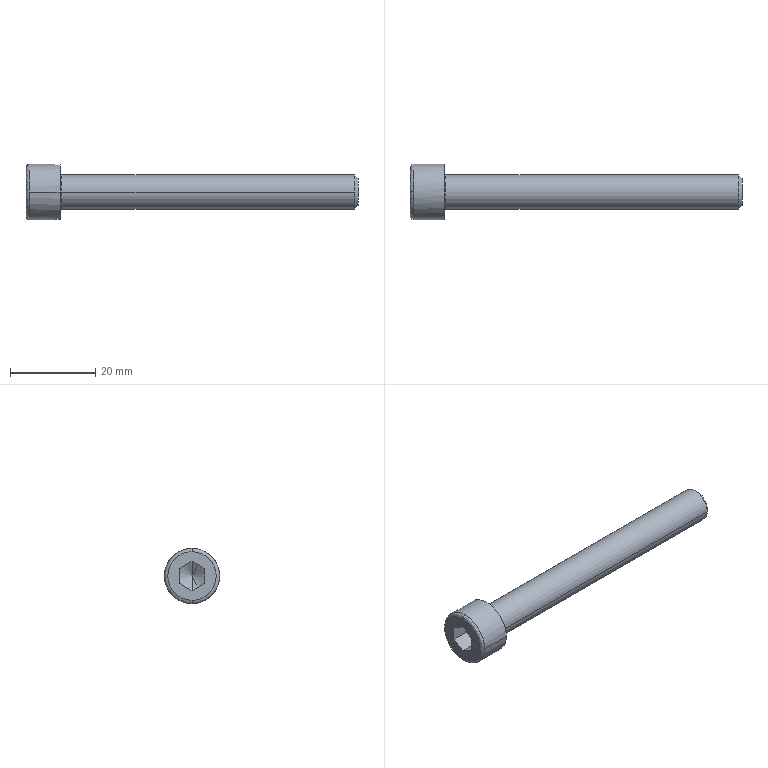Part | STEP file | Broached Socket Head Cap Screw - Metric M8x1.25 x 70 | 1 solid | 21 faces | box 78 x 13 x 13 mm | volume 4420 mm3 | plane 9 | spline 4 | cylinder 4 | cone 4 | commonest cylinder face diameters 8 x2 13 x2